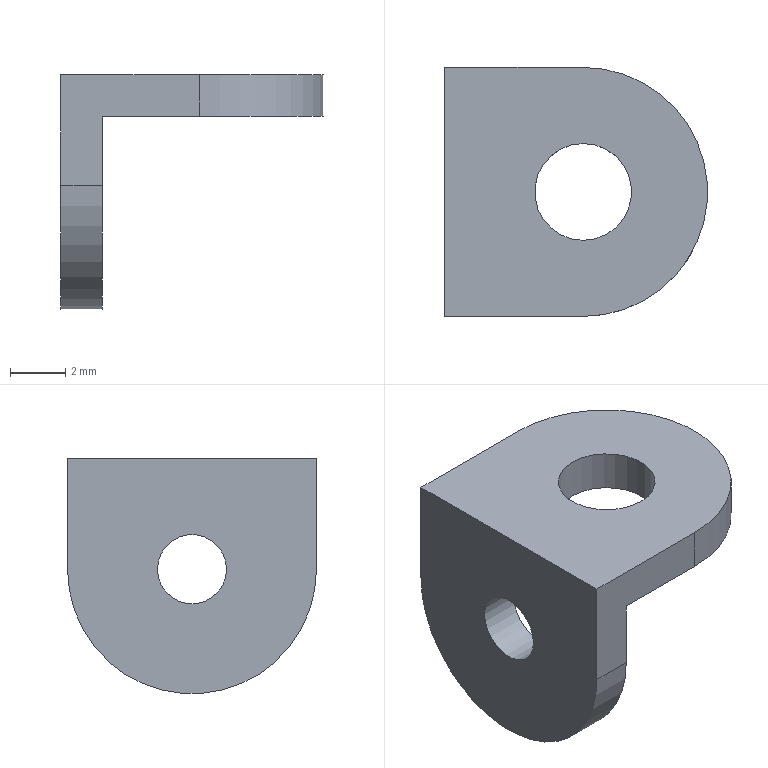Part | STEP file | 1-41.2 | 1 solid | 10 faces | box 9.5 x 9 x 8.5 mm | volume 174.881 mm3 | plane 6 | cylinder 4 | commonest cylinder face diameters 9 x2 2.5 x1 3.5 x1
STEP:
#1=CARTESIAN_POINT('',(0.,0.,0.));
#2=DIRECTION('',(0.,0.,1.));
#3=DIRECTION('',(1.,0.,0.));
#4=AXIS2_PLACEMENT_3D('',#1,#2,#3);
#5=CARTESIAN_POINT('',(0.,-4.5,1.5));
#6=VERTEX_POINT('',#5);
#7=CARTESIAN_POINT('',(0.,4.5,1.5));
#8=VERTEX_POINT('',#7);
#9=CARTESIAN_POINT('',(0.,0.,1.5));
#10=DIRECTION('',(0.,0.,1.));
#11=DIRECTION('',(0.,-1.,0.));
#12=AXIS2_PLACEMENT_3D('',#9,#10,#11);
#13=CIRCLE('',#12,4.5);
#14=CARTESIAN_POINT('',(-0.25,0.25,1.5));
#15=DIRECTION('',(0.,0.,1.));
#16=DIRECTION('',(0.,1.,0.));
#17=AXIS2_PLACEMENT_3D('',#14,#15,#16);
#18=PLANE('',#17);
#19=CARTESIAN_POINT('',(-0.25,-0.25));
#20=DIRECTION('',(-1.,0.));
#21=AXIS2_PLACEMENT_2D('',#19,#20);
#22=CIRCLE('',#21,4.5);
#23=(GEOMETRIC_REPRESENTATION_CONTEXT(2)PARAMETRIC_REPRESENTATION_CONTEXT()REPRESENTATION_CONTEXT('',''));
#24=DEFINITIONAL_REPRESENTATION('',(#22),#23);
#25=PCURVE('',#18,#24);
#26=CARTESIAN_POINT('',(0.,0.,0.));
#27=DIRECTION('',(0.,0.,1.));
#28=DIRECTION('',(0.,-1.,0.));
#29=AXIS2_PLACEMENT_3D('',#26,#27,#28);
#30=CYLINDRICAL_SURFACE('',#29,4.5);
#31=CARTESIAN_POINT('',(0.,1.5));
#32=DIRECTION('',(1.,0.));
#33=VECTOR('',#32,1.);
#34=LINE('',#31,#33);
#35=(GEOMETRIC_REPRESENTATION_CONTEXT(2)PARAMETRIC_REPRESENTATION_CONTEXT()REPRESENTATION_CONTEXT('',''));
#36=DEFINITIONAL_REPRESENTATION('',(#34),#35);
#37=PCURVE('',#30,#36);
#38=SURFACE_CURVE('',#13,(#25,#37),.PCURVE_S1.);
#39=EDGE_CURVE('',#6,#8,#38,.T.);
#40=ORIENTED_EDGE('',*,*,#39,.T.);
#41=CARTESIAN_POINT('',(-5.,4.5,1.5));
#42=VERTEX_POINT('',#41);
#43=CARTESIAN_POINT('',(0.,4.5,1.5));
#44=DIRECTION('',(-1.,0.,0.));
#45=VECTOR('',#44,1.);
#46=LINE('',#43,#45);
#47=CARTESIAN_POINT('',(4.25,-0.25));
#48=DIRECTION('',(0.,1.));
#49=VECTOR('',#48,1.);
#50=LINE('',#47,#49);
#51=(GEOMETRIC_REPRESENTATION_CONTEXT(2)PARAMETRIC_REPRESENTATION_CONTEXT()REPRESENTATION_CONTEXT('',''));
#52=DEFINITIONAL_REPRESENTATION('',(#50),#51);
#53=PCURVE('',#18,#52);
#54=CARTESIAN_POINT('',(-2.5,4.5,-0.5));
#55=DIRECTION('',(0.,1.,0.));
#56=DIRECTION('',(-1.,0.,0.));
#57=AXIS2_PLACEMENT_3D('',#54,#55,#56);
#58=PLANE('',#57);
#59=CARTESIAN_POINT('',(-2.5,2.));
#60=DIRECTION('',(1.,0.));
#61=VECTOR('',#60,1.);
#62=LINE('',#59,#61);
#63=(GEOMETRIC_REPRESENTATION_CONTEXT(2)PARAMETRIC_REPRESENTATION_CONTEXT()REPRESENTATION_CONTEXT('',''));
#64=DEFINITIONAL_REPRESENTATION('',(#62),#63);
#65=PCURVE('',#58,#64);
#66=SURFACE_CURVE('',#46,(#53,#65),.PCURVE_S1.);
#67=EDGE_CURVE('',#8,#42,#66,.T.);
#68=ORIENTED_EDGE('',*,*,#67,.T.);
#69=CARTESIAN_POINT('',(-5.,-4.5,1.5));
#70=VERTEX_POINT('',#69);
#71=CARTESIAN_POINT('',(-5.,4.5,1.5));
#72=DIRECTION('',(0.,-1.,0.));
#73=VECTOR('',#72,1.);
#74=LINE('',#71,#73);
#75=CARTESIAN_POINT('',(4.25,4.75));
#76=DIRECTION('',(-1.,0.));
#77=VECTOR('',#76,1.);
#78=LINE('',#75,#77);
#79=(GEOMETRIC_REPRESENTATION_CONTEXT(2)PARAMETRIC_REPRESENTATION_CONTEXT()REPRESENTATION_CONTEXT('',''));
#80=DEFINITIONAL_REPRESENTATION('',(#78),#79);
#81=PCURVE('',#18,#80);
#82=CARTESIAN_POINT('',(-5.,0.,-2.5));
#83=DIRECTION('',(-1.,0.,0.));
#84=DIRECTION('',(0.,-1.,0.));
#85=AXIS2_PLACEMENT_3D('',#82,#83,#84);
#86=PLANE('',#85);
#87=CARTESIAN_POINT('',(-4.5,4.));
#88=DIRECTION('',(1.,0.));
#89=VECTOR('',#88,1.);
#90=LINE('',#87,#89);
#91=(GEOMETRIC_REPRESENTATION_CONTEXT(2)PARAMETRIC_REPRESENTATION_CONTEXT()REPRESENTATION_CONTEXT('',''));
#92=DEFINITIONAL_REPRESENTATION('',(#90),#91);
#93=PCURVE('',#86,#92);
#94=SURFACE_CURVE('',#74,(#81,#93),.PCURVE_S1.);
#95=EDGE_CURVE('',#42,#70,#94,.T.);
#96=ORIENTED_EDGE('',*,*,#95,.T.);
#97=CARTESIAN_POINT('',(-5.,-4.5,1.5));
#98=DIRECTION('',(1.,0.,0.));
#99=VECTOR('',#98,1.);
#100=LINE('',#97,#99);
#101=CARTESIAN_POINT('',(-4.75,4.75));
#102=DIRECTION('',(0.,-1.));
#103=VECTOR('',#102,1.);
#104=LINE('',#101,#103);
#105=(GEOMETRIC_REPRESENTATION_CONTEXT(2)PARAMETRIC_REPRESENTATION_CONTEXT()REPRESENTATION_CONTEXT('',''));
#106=DEFINITIONAL_REPRESENTATION('',(#104),#105);
#107=PCURVE('',#18,#106);
#108=CARTESIAN_POINT('',(-2.5,-4.5,-0.5));
#109=DIRECTION('',(0.,-1.,0.));
#110=DIRECTION('',(1.,0.,0.));
#111=AXIS2_PLACEMENT_3D('',#108,#109,#110);
#112=PLANE('',#111);
#113=CARTESIAN_POINT('',(-2.5,2.));
#114=DIRECTION('',(1.,0.));
#115=VECTOR('',#114,1.);
#116=LINE('',#113,#115);
#117=(GEOMETRIC_REPRESENTATION_CONTEXT(2)PARAMETRIC_REPRESENTATION_CONTEXT()REPRESENTATION_CONTEXT('',''));
#118=DEFINITIONAL_REPRESENTATION('',(#116),#117);
#119=PCURVE('',#112,#118);
#120=SURFACE_CURVE('',#100,(#107,#119),.PCURVE_S1.);
#121=EDGE_CURVE('',#70,#6,#120,.T.);
#122=ORIENTED_EDGE('',*,*,#121,.T.);
#123=EDGE_LOOP('',(#40,#68,#96,#122));
#124=FACE_BOUND('',#123,.T.);
#125=CARTESIAN_POINT('',(0.,1.75,1.5));
#126=VERTEX_POINT('',#125);
#127=CARTESIAN_POINT('',(0.,0.,1.5));
#128=DIRECTION('',(0.,0.,-1.));
#129=DIRECTION('',(0.,1.,0.));
#130=AXIS2_PLACEMENT_3D('',#127,#128,#129);
#131=CIRCLE('',#130,1.75);
#132=CARTESIAN_POINT('',(1.5,-0.25));
#133=CARTESIAN_POINT('',(1.5,-3.281));
#134=CARTESIAN_POINT('',(-1.125,-1.766));
#135=CARTESIAN_POINT('',(-3.75,-0.25));
#136=CARTESIAN_POINT('',(-1.125,1.266));
#137=CARTESIAN_POINT('',(1.5,2.781));
#138=CARTESIAN_POINT('',(1.5,-0.25));
#139=(BOUNDED_CURVE()B_SPLINE_CURVE(2,(#132,#133,#134,#135,#136,#137,#138),.UNSPECIFIED.,.T.,.F.)B_SPLINE_CURVE_WITH_KNOTS((1,2,2,2,2,1),(-2.094,0.,2.094,4.189,6.283,8.378),.UNSPECIFIED.)CURVE()GEOMETRIC_REPRESENTATION_ITEM()RATIONAL_B_SPLINE_CURVE((1.,0.5,1.,0.5,1.,0.5,1.))REPRESENTATION_ITEM(''));
#140=(GEOMETRIC_REPRESENTATION_CONTEXT(2)PARAMETRIC_REPRESENTATION_CONTEXT()REPRESENTATION_CONTEXT('',''));
#141=DEFINITIONAL_REPRESENTATION('',(#139),#140);
#142=PCURVE('',#18,#141);
#143=CARTESIAN_POINT('',(0.,0.,0.));
#144=DIRECTION('',(0.,0.,1.));
#145=DIRECTION('',(0.,1.,0.));
#146=AXIS2_PLACEMENT_3D('',#143,#144,#145);
#147=CYLINDRICAL_SURFACE('',#146,1.75);
#148=CARTESIAN_POINT('',(6.283,1.5));
#149=DIRECTION('',(-1.,0.));
#150=VECTOR('',#149,1.);
#151=LINE('',#148,#150);
#152=(GEOMETRIC_REPRESENTATION_CONTEXT(2)PARAMETRIC_REPRESENTATION_CONTEXT()REPRESENTATION_CONTEXT('',''));
#153=DEFINITIONAL_REPRESENTATION('',(#151),#152);
#154=PCURVE('',#147,#153);
#155=SURFACE_CURVE('',#131,(#142,#154),.PCURVE_S1.);
#156=EDGE_CURVE('',#126,#126,#155,.T.);
#157=ORIENTED_EDGE('',*,*,#156,.T.);
#158=EDGE_LOOP('',(#157));
#159=FACE_BOUND('',#158,.T.);
#160=ADVANCED_FACE('',(#124,#159),#18,.T.);
#161=CARTESIAN_POINT('',(0.,-4.5,0.));
#162=VERTEX_POINT('',#161);
#163=CARTESIAN_POINT('',(0.,4.5,0.));
#164=VERTEX_POINT('',#163);
#165=CARTESIAN_POINT('',(0.,0.,0.));
#166=DIRECTION('',(0.,0.,1.));
#167=DIRECTION('',(0.,-1.,0.));
#168=AXIS2_PLACEMENT_3D('',#165,#166,#167);
#169=CIRCLE('',#168,4.5);
#170=CARTESIAN_POINT('',(0.,0.));
#171=DIRECTION('',(1.,0.));
#172=VECTOR('',#171,1.);
#173=LINE('',#170,#172);
#174=(GEOMETRIC_REPRESENTATION_CONTEXT(2)PARAMETRIC_REPRESENTATION_CONTEXT()REPRESENTATION_CONTEXT('',''));
#175=DEFINITIONAL_REPRESENTATION('',(#173),#174);
#176=PCURVE('',#30,#175);
#177=CARTESIAN_POINT('',(-0.25,0.25,0.));
#178=DIRECTION('',(0.,0.,1.));
#179=DIRECTION('',(0.,1.,0.));
#180=AXIS2_PLACEMENT_3D('',#177,#178,#179);
#181=PLANE('',#180);
#182=CARTESIAN_POINT('',(-0.25,-0.25));
#183=DIRECTION('',(-1.,0.));
#184=AXIS2_PLACEMENT_2D('',#182,#183);
#185=CIRCLE('',#184,4.5);
#186=(GEOMETRIC_REPRESENTATION_CONTEXT(2)PARAMETRIC_REPRESENTATION_CONTEXT()REPRESENTATION_CONTEXT('',''));
#187=DEFINITIONAL_REPRESENTATION('',(#185),#186);
#188=PCURVE('',#181,#187);
#189=SURFACE_CURVE('',#169,(#176,#188),.PCURVE_S1.);
#190=EDGE_CURVE('',#162,#164,#189,.T.);
#191=ORIENTED_EDGE('',*,*,#190,.T.);
#192=CARTESIAN_POINT('',(0.,4.5,0.));
#193=DIRECTION('',(0.,0.,1.));
#194=VECTOR('',#193,1.);
#195=LINE('',#192,#194);
#196=CARTESIAN_POINT('',(3.142,0.));
#197=DIRECTION('',(0.,1.));
#198=VECTOR('',#197,1.);
#199=LINE('',#196,#198);
#200=(GEOMETRIC_REPRESENTATION_CONTEXT(2)PARAMETRIC_REPRESENTATION_CONTEXT()REPRESENTATION_CONTEXT('',''));
#201=DEFINITIONAL_REPRESENTATION('',(#199),#200);
#202=PCURVE('',#30,#201);
#203=CARTESIAN_POINT('',(-2.5,0.5));
#204=DIRECTION('',(0.,1.));
#205=VECTOR('',#204,1.);
#206=LINE('',#203,#205);
#207=(GEOMETRIC_REPRESENTATION_CONTEXT(2)PARAMETRIC_REPRESENTATION_CONTEXT()REPRESENTATION_CONTEXT('',''));
#208=DEFINITIONAL_REPRESENTATION('',(#206),#207);
#209=PCURVE('',#58,#208);
#210=SURFACE_CURVE('',#195,(#202,#209),.PCURVE_S1.);
#211=EDGE_CURVE('',#164,#8,#210,.T.);
#212=ORIENTED_EDGE('',*,*,#211,.T.);
#213=ORIENTED_EDGE('',*,*,#39,.F.);
#214=CARTESIAN_POINT('',(0.,-4.5,0.));
#215=DIRECTION('',(0.,0.,1.));
#216=VECTOR('',#215,1.);
#217=LINE('',#214,#216);
#218=CARTESIAN_POINT('',(0.,0.));
#219=DIRECTION('',(0.,1.));
#220=VECTOR('',#219,1.);
#221=LINE('',#218,#220);
#222=(GEOMETRIC_REPRESENTATION_CONTEXT(2)PARAMETRIC_REPRESENTATION_CONTEXT()REPRESENTATION_CONTEXT('',''));
#223=DEFINITIONAL_REPRESENTATION('',(#221),#222);
#224=PCURVE('',#30,#223);
#225=CARTESIAN_POINT('',(2.5,0.5));
#226=DIRECTION('',(0.,1.));
#227=VECTOR('',#226,1.);
#228=LINE('',#225,#227);
#229=(GEOMETRIC_REPRESENTATION_CONTEXT(2)PARAMETRIC_REPRESENTATION_CONTEXT()REPRESENTATION_CONTEXT('',''));
#230=DEFINITIONAL_REPRESENTATION('',(#228),#229);
#231=PCURVE('',#112,#230);
#232=SURFACE_CURVE('',#217,(#224,#231),.PCURVE_S1.);
#233=EDGE_CURVE('',#162,#6,#232,.T.);
#234=ORIENTED_EDGE('',*,*,#233,.F.);
#235=EDGE_LOOP('',(#191,#212,#213,#234));
#236=FACE_BOUND('',#235,.T.);
#237=ADVANCED_FACE('',(#236),#30,.T.);
#238=ORIENTED_EDGE('',*,*,#67,.F.);
#239=ORIENTED_EDGE('',*,*,#211,.F.);
#240=CARTESIAN_POINT('',(-3.5,4.5,0.));
#241=VERTEX_POINT('',#240);
#242=CARTESIAN_POINT('',(0.,4.5,0.));
#243=DIRECTION('',(-1.,0.,0.));
#244=VECTOR('',#243,1.);
#245=LINE('',#242,#244);
#246=CARTESIAN_POINT('',(-2.5,0.5));
#247=DIRECTION('',(1.,0.));
#248=VECTOR('',#247,1.);
#249=LINE('',#246,#248);
#250=(GEOMETRIC_REPRESENTATION_CONTEXT(2)PARAMETRIC_REPRESENTATION_CONTEXT()REPRESENTATION_CONTEXT('',''));
#251=DEFINITIONAL_REPRESENTATION('',(#249),#250);
#252=PCURVE('',#58,#251);
#253=CARTESIAN_POINT('',(4.25,-0.25));
#254=DIRECTION('',(0.,1.));
#255=VECTOR('',#254,1.);
#256=LINE('',#253,#255);
#257=(GEOMETRIC_REPRESENTATION_CONTEXT(2)PARAMETRIC_REPRESENTATION_CONTEXT()REPRESENTATION_CONTEXT('',''));
#258=DEFINITIONAL_REPRESENTATION('',(#256),#257);
#259=PCURVE('',#181,#258);
#260=SURFACE_CURVE('',#245,(#252,#259),.PCURVE_S1.);
#261=EDGE_CURVE('',#164,#241,#260,.T.);
#262=ORIENTED_EDGE('',*,*,#261,.T.);
#263=CARTESIAN_POINT('',(-3.5,4.5,-2.5));
#264=VERTEX_POINT('',#263);
#265=CARTESIAN_POINT('',(-3.5,4.5,0.));
#266=DIRECTION('',(0.,0.,-1.));
#267=VECTOR('',#266,1.);
#268=LINE('',#265,#267);
#269=CARTESIAN_POINT('',(1.,0.5));
#270=DIRECTION('',(0.,-1.));
#271=VECTOR('',#270,1.);
#272=LINE('',#269,#271);
#273=(GEOMETRIC_REPRESENTATION_CONTEXT(2)PARAMETRIC_REPRESENTATION_CONTEXT()REPRESENTATION_CONTEXT('',''));
#274=DEFINITIONAL_REPRESENTATION('',(#272),#273);
#275=PCURVE('',#58,#274);
#276=CARTESIAN_POINT('',(-3.5,0.,-2.5));
#277=DIRECTION('',(-1.,0.,0.));
#278=DIRECTION('',(0.,-1.,0.));
#279=AXIS2_PLACEMENT_3D('',#276,#277,#278);
#280=PLANE('',#279);
#281=CARTESIAN_POINT('',(-4.5,2.5));
#282=DIRECTION('',(0.,-1.));
#283=VECTOR('',#282,1.);
#284=LINE('',#281,#283);
#285=(GEOMETRIC_REPRESENTATION_CONTEXT(2)PARAMETRIC_REPRESENTATION_CONTEXT()REPRESENTATION_CONTEXT('',''));
#286=DEFINITIONAL_REPRESENTATION('',(#284),#285);
#287=PCURVE('',#280,#286);
#288=SURFACE_CURVE('',#268,(#275,#287),.PCURVE_S1.);
#289=EDGE_CURVE('',#241,#264,#288,.T.);
#290=ORIENTED_EDGE('',*,*,#289,.T.);
#291=CARTESIAN_POINT('',(-5.,4.5,-2.5));
#292=VERTEX_POINT('',#291);
#293=CARTESIAN_POINT('',(-5.,4.5,-2.5));
#294=DIRECTION('',(1.,0.,0.));
#295=VECTOR('',#294,1.);
#296=LINE('',#293,#295);
#297=CARTESIAN_POINT('',(2.5,-2.));
#298=DIRECTION('',(-1.,0.));
#299=VECTOR('',#298,1.);
#300=LINE('',#297,#299);
#301=(GEOMETRIC_REPRESENTATION_CONTEXT(2)PARAMETRIC_REPRESENTATION_CONTEXT()REPRESENTATION_CONTEXT('',''));
#302=DEFINITIONAL_REPRESENTATION('',(#300),#301);
#303=PCURVE('',#58,#302);
#304=CARTESIAN_POINT('',(-5.,0.,-2.5));
#305=DIRECTION('',(1.,0.,0.));
#306=DIRECTION('',(0.,1.,0.));
#307=AXIS2_PLACEMENT_3D('',#304,#305,#306);
#308=CYLINDRICAL_SURFACE('',#307,4.5);
#309=CARTESIAN_POINT('',(6.283,0.));
#310=DIRECTION('',(0.,1.));
#311=VECTOR('',#310,1.);
#312=LINE('',#309,#311);
#313=(GEOMETRIC_REPRESENTATION_CONTEXT(2)PARAMETRIC_REPRESENTATION_CONTEXT()REPRESENTATION_CONTEXT('',''));
#314=DEFINITIONAL_REPRESENTATION('',(#312),#313);
#315=PCURVE('',#308,#314);
#316=SURFACE_CURVE('',#296,(#303,#315),.PCURVE_S1.);
#317=EDGE_CURVE('',#292,#264,#316,.T.);
#318=ORIENTED_EDGE('',*,*,#317,.F.);
#319=CARTESIAN_POINT('',(-5.,4.5,-2.5));
#320=DIRECTION('',(0.,0.,1.));
#321=VECTOR('',#320,1.);
#322=LINE('',#319,#321);
#323=CARTESIAN_POINT('',(2.5,-2.));
#324=DIRECTION('',(0.,1.));
#325=VECTOR('',#324,1.);
#326=LINE('',#323,#325);
#327=(GEOMETRIC_REPRESENTATION_CONTEXT(2)PARAMETRIC_REPRESENTATION_CONTEXT()REPRESENTATION_CONTEXT('',''));
#328=DEFINITIONAL_REPRESENTATION('',(#326),#327);
#329=PCURVE('',#58,#328);
#330=CARTESIAN_POINT('',(-4.5,0.));
#331=DIRECTION('',(0.,1.));
#332=VECTOR('',#331,1.);
#333=LINE('',#330,#332);
#334=(GEOMETRIC_REPRESENTATION_CONTEXT(2)PARAMETRIC_REPRESENTATION_CONTEXT()REPRESENTATION_CONTEXT('',''));
#335=DEFINITIONAL_REPRESENTATION('',(#333),#334);
#336=PCURVE('',#86,#335);
#337=SURFACE_CURVE('',#322,(#329,#336),.PCURVE_S1.);
#338=EDGE_CURVE('',#292,#42,#337,.T.);
#339=ORIENTED_EDGE('',*,*,#338,.T.);
#340=EDGE_LOOP('',(#238,#239,#262,#290,#318,#339));
#341=FACE_BOUND('',#340,.T.);
#342=ADVANCED_FACE('',(#341),#58,.T.);
#343=ORIENTED_EDGE('',*,*,#95,.F.);
#344=ORIENTED_EDGE('',*,*,#338,.F.);
#345=CARTESIAN_POINT('',(-5.,-4.5,-2.5));
#346=VERTEX_POINT('',#345);
#347=CARTESIAN_POINT('',(-5.,0.,-2.5));
#348=DIRECTION('',(-1.,0.,0.));
#349=DIRECTION('',(0.,1.,0.));
#350=AXIS2_PLACEMENT_3D('',#347,#348,#349);
#351=CIRCLE('',#350,4.5);
#352=CARTESIAN_POINT('',(0.,0.));
#353=DIRECTION('',(-1.,0.));
#354=AXIS2_PLACEMENT_2D('',#352,#353);
#355=CIRCLE('',#354,4.5);
#356=(GEOMETRIC_REPRESENTATION_CONTEXT(2)PARAMETRIC_REPRESENTATION_CONTEXT()REPRESENTATION_CONTEXT('',''));
#357=DEFINITIONAL_REPRESENTATION('',(#355),#356);
#358=PCURVE('',#86,#357);
#359=CARTESIAN_POINT('',(6.283,0.));
#360=DIRECTION('',(-1.,0.));
#361=VECTOR('',#360,1.);
#362=LINE('',#359,#361);
#363=(GEOMETRIC_REPRESENTATION_CONTEXT(2)PARAMETRIC_REPRESENTATION_CONTEXT()REPRESENTATION_CONTEXT('',''));
#364=DEFINITIONAL_REPRESENTATION('',(#362),#363);
#365=PCURVE('',#308,#364);
#366=SURFACE_CURVE('',#351,(#358,#365),.PCURVE_S1.);
#367=EDGE_CURVE('',#292,#346,#366,.T.);
#368=ORIENTED_EDGE('',*,*,#367,.T.);
#369=CARTESIAN_POINT('',(-5.,-4.5,1.5));
#370=DIRECTION('',(0.,0.,-1.));
#371=VECTOR('',#370,1.);
#372=LINE('',#369,#371);
#373=CARTESIAN_POINT('',(4.5,4.));
#374=DIRECTION('',(0.,-1.));
#375=VECTOR('',#374,1.);
#376=LINE('',#373,#375);
#377=(GEOMETRIC_REPRESENTATION_CONTEXT(2)PARAMETRIC_REPRESENTATION_CONTEXT()REPRESENTATION_CONTEXT('',''));
#378=DEFINITIONAL_REPRESENTATION('',(#376),#377);
#379=PCURVE('',#86,#378);
#380=CARTESIAN_POINT('',(-2.5,2.));
#381=DIRECTION('',(0.,-1.));
#382=VECTOR('',#381,1.);
#383=LINE('',#380,#382);
#384=(GEOMETRIC_REPRESENTATION_CONTEXT(2)PARAMETRIC_REPRESENTATION_CONTEXT()REPRESENTATION_CONTEXT('',''));
#385=DEFINITIONAL_REPRESENTATION('',(#383),#384);
#386=PCURVE('',#112,#385);
#387=SURFACE_CURVE('',#372,(#379,#386),.PCURVE_S1.);
#388=EDGE_CURVE('',#70,#346,#387,.T.);
#389=ORIENTED_EDGE('',*,*,#388,.F.);
#390=EDGE_LOOP('',(#343,#344,#368,#389));
#391=FACE_BOUND('',#390,.T.);
#392=CARTESIAN_POINT('',(-5.,-1.25,-2.5));
#393=VERTEX_POINT('',#392);
#394=CARTESIAN_POINT('',(-5.,0.,-2.5));
#395=DIRECTION('',(1.,0.,0.));
#396=DIRECTION('',(0.,-1.,0.));
#397=AXIS2_PLACEMENT_3D('',#394,#395,#396);
#398=CIRCLE('',#397,1.25);
#399=CARTESIAN_POINT('',(1.25,0.));
#400=CARTESIAN_POINT('',(1.25,-2.165));
#401=CARTESIAN_POINT('',(-0.625,-1.083));
#402=CARTESIAN_POINT('',(-2.5,0.));
#403=CARTESIAN_POINT('',(-0.625,1.083));
#404=CARTESIAN_POINT('',(1.25,2.165));
#405=CARTESIAN_POINT('',(1.25,0.));
#406=(BOUNDED_CURVE()B_SPLINE_CURVE(2,(#399,#400,#401,#402,#403,#404,#405),.UNSPECIFIED.,.T.,.F.)B_SPLINE_CURVE_WITH_KNOTS((1,2,2,2,2,1),(-2.094,0.,2.094,4.189,6.283,8.378),.UNSPECIFIED.)CURVE()GEOMETRIC_REPRESENTATION_ITEM()RATIONAL_B_SPLINE_CURVE((1.,0.5,1.,0.5,1.,0.5,1.))REPRESENTATION_ITEM(''));
#407=(GEOMETRIC_REPRESENTATION_CONTEXT(2)PARAMETRIC_REPRESENTATION_CONTEXT()REPRESENTATION_CONTEXT('',''));
#408=DEFINITIONAL_REPRESENTATION('',(#406),#407);
#409=PCURVE('',#86,#408);
#410=CARTESIAN_POINT('',(-5.,0.,-2.5));
#411=DIRECTION('',(1.,0.,0.));
#412=DIRECTION('',(0.,-1.,0.));
#413=AXIS2_PLACEMENT_3D('',#410,#411,#412);
#414=CYLINDRICAL_SURFACE('',#413,1.25);
#415=CARTESIAN_POINT('',(0.,0.));
#416=DIRECTION('',(1.,0.));
#417=VECTOR('',#416,1.);
#418=LINE('',#415,#417);
#419=(GEOMETRIC_REPRESENTATION_CONTEXT(2)PARAMETRIC_REPRESENTATION_CONTEXT()REPRESENTATION_CONTEXT('',''));
#420=DEFINITIONAL_REPRESENTATION('',(#418),#419);
#421=PCURVE('',#414,#420);
#422=SURFACE_CURVE('',#398,(#409,#421),.PCURVE_S1.);
#423=EDGE_CURVE('',#393,#393,#422,.T.);
#424=ORIENTED_EDGE('',*,*,#423,.T.);
#425=EDGE_LOOP('',(#424));
#426=FACE_BOUND('',#425,.T.);
#427=ADVANCED_FACE('',(#391,#426),#86,.T.);
#428=CARTESIAN_POINT('',(-3.5,-4.5,0.));
#429=VERTEX_POINT('',#428);
#430=CARTESIAN_POINT('',(-3.5,-4.5,0.));
#431=DIRECTION('',(1.,0.,0.));
#432=VECTOR('',#431,1.);
#433=LINE('',#430,#432);
#434=CARTESIAN_POINT('',(-1.,0.5));
#435=DIRECTION('',(1.,0.));
#436=VECTOR('',#435,1.);
#437=LINE('',#434,#436);
#438=(GEOMETRIC_REPRESENTATION_CONTEXT(2)PARAMETRIC_REPRESENTATION_CONTEXT()REPRESENTATION_CONTEXT('',''));
#439=DEFINITIONAL_REPRESENTATION('',(#437),#438);
#440=PCURVE('',#112,#439);
#441=CARTESIAN_POINT('',(-4.75,3.25));
#442=DIRECTION('',(0.,-1.));
#443=VECTOR('',#442,1.);
#444=LINE('',#441,#443);
#445=(GEOMETRIC_REPRESENTATION_CONTEXT(2)PARAMETRIC_REPRESENTATION_CONTEXT()REPRESENTATION_CONTEXT('',''));
#446=DEFINITIONAL_REPRESENTATION('',(#444),#445);
#447=PCURVE('',#181,#446);
#448=SURFACE_CURVE('',#433,(#440,#447),.PCURVE_S1.);
#449=EDGE_CURVE('',#429,#162,#448,.T.);
#450=ORIENTED_EDGE('',*,*,#449,.T.);
#451=ORIENTED_EDGE('',*,*,#233,.T.);
#452=ORIENTED_EDGE('',*,*,#121,.F.);
#453=ORIENTED_EDGE('',*,*,#388,.T.);
#454=CARTESIAN_POINT('',(-3.5,-4.5,-2.5));
#455=VERTEX_POINT('',#454);
#456=CARTESIAN_POINT('',(-5.,-4.5,-2.5));
#457=DIRECTION('',(1.,0.,0.));
#458=VECTOR('',#457,1.);
#459=LINE('',#456,#458);
#460=CARTESIAN_POINT('',(-2.5,-2.));
#461=DIRECTION('',(1.,0.));
#462=VECTOR('',#461,1.);
#463=LINE('',#460,#462);
#464=(GEOMETRIC_REPRESENTATION_CONTEXT(2)PARAMETRIC_REPRESENTATION_CONTEXT()REPRESENTATION_CONTEXT('',''));
#465=DEFINITIONAL_REPRESENTATION('',(#463),#464);
#466=PCURVE('',#112,#465);
#467=CARTESIAN_POINT('',(3.142,0.));
#468=DIRECTION('',(0.,1.));
#469=VECTOR('',#468,1.);
#470=LINE('',#467,#469);
#471=(GEOMETRIC_REPRESENTATION_CONTEXT(2)PARAMETRIC_REPRESENTATION_CONTEXT()REPRESENTATION_CONTEXT('',''));
#472=DEFINITIONAL_REPRESENTATION('',(#470),#471);
#473=PCURVE('',#308,#472);
#474=SURFACE_CURVE('',#459,(#466,#473),.PCURVE_S1.);
#475=EDGE_CURVE('',#346,#455,#474,.T.);
#476=ORIENTED_EDGE('',*,*,#475,.T.);
#477=CARTESIAN_POINT('',(-3.5,-4.5,-2.5));
#478=DIRECTION('',(0.,0.,1.));
#479=VECTOR('',#478,1.);
#480=LINE('',#477,#479);
#481=CARTESIAN_POINT('',(-1.,-2.));
#482=DIRECTION('',(0.,1.));
#483=VECTOR('',#482,1.);
#484=LINE('',#481,#483);
#485=(GEOMETRIC_REPRESENTATION_CONTEXT(2)PARAMETRIC_REPRESENTATION_CONTEXT()REPRESENTATION_CONTEXT('',''));
#486=DEFINITIONAL_REPRESENTATION('',(#484),#485);
#487=PCURVE('',#112,#486);
#488=CARTESIAN_POINT('',(4.5,0.));
#489=DIRECTION('',(0.,1.));
#490=VECTOR('',#489,1.);
#491=LINE('',#488,#490);
#492=(GEOMETRIC_REPRESENTATION_CONTEXT(2)PARAMETRIC_REPRESENTATION_CONTEXT()REPRESENTATION_CONTEXT('',''));
#493=DEFINITIONAL_REPRESENTATION('',(#491),#492);
#494=PCURVE('',#280,#493);
#495=SURFACE_CURVE('',#480,(#487,#494),.PCURVE_S1.);
#496=EDGE_CURVE('',#455,#429,#495,.T.);
#497=ORIENTED_EDGE('',*,*,#496,.T.);
#498=EDGE_LOOP('',(#450,#451,#452,#453,#476,#497));
#499=FACE_BOUND('',#498,.T.);
#500=ADVANCED_FACE('',(#499),#112,.T.);
#501=CARTESIAN_POINT('',(0.,1.75,0.));
#502=VERTEX_POINT('',#501);
#503=CARTESIAN_POINT('',(0.,1.75,0.));
#504=DIRECTION('',(0.,0.,1.));
#505=VECTOR('',#504,1.);
#506=LINE('',#503,#505);
#507=CARTESIAN_POINT('',(6.283,0.));
#508=DIRECTION('',(0.,1.));
#509=VECTOR('',#508,1.);
#510=LINE('',#507,#509);
#511=(GEOMETRIC_REPRESENTATION_CONTEXT(2)PARAMETRIC_REPRESENTATION_CONTEXT()REPRESENTATION_CONTEXT('',''));
#512=DEFINITIONAL_REPRESENTATION('',(#510),#511);
#513=PCURVE('',#147,#512);
#514=CARTESIAN_POINT('',(0.,0.));
#515=DIRECTION('',(0.,1.));
#516=VECTOR('',#515,1.);
#517=LINE('',#514,#516);
#518=(GEOMETRIC_REPRESENTATION_CONTEXT(2)PARAMETRIC_REPRESENTATION_CONTEXT()REPRESENTATION_CONTEXT('',''));
#519=DEFINITIONAL_REPRESENTATION('',(#517),#518);
#520=PCURVE('',#147,#519);
#521=SEAM_CURVE('',#506,(#513,#520),.PCURVE_S1.);
#522=EDGE_CURVE('',#502,#126,#521,.T.);
#523=ORIENTED_EDGE('',*,*,#522,.T.);
#524=ORIENTED_EDGE('',*,*,#156,.T.);
#525=ORIENTED_EDGE('',*,*,#522,.F.);
#526=CARTESIAN_POINT('',(0.,0.,0.));
#527=DIRECTION('',(0.,0.,-1.));
#528=DIRECTION('',(0.,1.,0.));
#529=AXIS2_PLACEMENT_3D('',#526,#527,#528);
#530=CIRCLE('',#529,1.75);
#531=CARTESIAN_POINT('',(6.283,0.));
#532=DIRECTION('',(-1.,0.));
#533=VECTOR('',#532,1.);
#534=LINE('',#531,#533);
#535=(GEOMETRIC_REPRESENTATION_CONTEXT(2)PARAMETRIC_REPRESENTATION_CONTEXT()REPRESENTATION_CONTEXT('',''));
#536=DEFINITIONAL_REPRESENTATION('',(#534),#535);
#537=PCURVE('',#147,#536);
#538=CARTESIAN_POINT('',(1.5,-0.25));
#539=CARTESIAN_POINT('',(1.5,-3.281));
#540=CARTESIAN_POINT('',(-1.125,-1.766));
#541=CARTESIAN_POINT('',(-3.75,-0.25));
#542=CARTESIAN_POINT('',(-1.125,1.266));
#543=CARTESIAN_POINT('',(1.5,2.781));
#544=CARTESIAN_POINT('',(1.5,-0.25));
#545=(BOUNDED_CURVE()B_SPLINE_CURVE(2,(#538,#539,#540,#541,#542,#543,#544),.UNSPECIFIED.,.T.,.F.)B_SPLINE_CURVE_WITH_KNOTS((1,2,2,2,2,1),(-2.094,0.,2.094,4.189,6.283,8.378),.UNSPECIFIED.)CURVE()GEOMETRIC_REPRESENTATION_ITEM()RATIONAL_B_SPLINE_CURVE((1.,0.5,1.,0.5,1.,0.5,1.))REPRESENTATION_ITEM(''));
#546=(GEOMETRIC_REPRESENTATION_CONTEXT(2)PARAMETRIC_REPRESENTATION_CONTEXT()REPRESENTATION_CONTEXT('',''));
#547=DEFINITIONAL_REPRESENTATION('',(#545),#546);
#548=PCURVE('',#181,#547);
#549=SURFACE_CURVE('',#530,(#537,#548),.PCURVE_S1.);
#550=EDGE_CURVE('',#502,#502,#549,.T.);
#551=ORIENTED_EDGE('',*,*,#550,.F.);
#552=EDGE_LOOP('',(#523,#524,#525,#551));
#553=FACE_BOUND('',#552,.F.);
#554=ADVANCED_FACE('',(#553),#147,.F.);
#555=ORIENTED_EDGE('',*,*,#190,.T.);
#556=ORIENTED_EDGE('',*,*,#261,.T.);
#557=CARTESIAN_POINT('',(-3.5,-4.5,0.));
#558=DIRECTION('',(0.,1.,0.));
#559=VECTOR('',#558,1.);
#560=LINE('',#557,#559);
#561=CARTESIAN_POINT('',(-4.75,3.25));
#562=DIRECTION('',(1.,0.));
#563=VECTOR('',#562,1.);
#564=LINE('',#561,#563);
#565=(GEOMETRIC_REPRESENTATION_CONTEXT(2)PARAMETRIC_REPRESENTATION_CONTEXT()REPRESENTATION_CONTEXT('',''));
#566=DEFINITIONAL_REPRESENTATION('',(#564),#565);
#567=PCURVE('',#181,#566);
#568=CARTESIAN_POINT('',(4.5,2.5));
#569=DIRECTION('',(-1.,0.));
#570=VECTOR('',#569,1.);
#571=LINE('',#568,#570);
#572=(GEOMETRIC_REPRESENTATION_CONTEXT(2)PARAMETRIC_REPRESENTATION_CONTEXT()REPRESENTATION_CONTEXT('',''));
#573=DEFINITIONAL_REPRESENTATION('',(#571),#572);
#574=PCURVE('',#280,#573);
#575=SURFACE_CURVE('',#560,(#567,#574),.PCURVE_S1.);
#576=EDGE_CURVE('',#429,#241,#575,.T.);
#577=ORIENTED_EDGE('',*,*,#576,.F.);
#578=ORIENTED_EDGE('',*,*,#449,.T.);
#579=EDGE_LOOP('',(#555,#556,#577,#578));
#580=FACE_BOUND('',#579,.F.);
#581=ORIENTED_EDGE('',*,*,#550,.T.);
#582=EDGE_LOOP('',(#581));
#583=FACE_BOUND('',#582,.F.);
#584=ADVANCED_FACE('',(#580,#583),#181,.F.);
#585=CARTESIAN_POINT('',(-3.5,0.,-2.5));
#586=DIRECTION('',(-1.,0.,0.));
#587=DIRECTION('',(0.,1.,0.));
#588=AXIS2_PLACEMENT_3D('',#585,#586,#587);
#589=CIRCLE('',#588,4.5);
#590=CARTESIAN_POINT('',(0.,0.));
#591=DIRECTION('',(-1.,0.));
#592=AXIS2_PLACEMENT_2D('',#590,#591);
#593=CIRCLE('',#592,4.5);
#594=(GEOMETRIC_REPRESENTATION_CONTEXT(2)PARAMETRIC_REPRESENTATION_CONTEXT()REPRESENTATION_CONTEXT('',''));
#595=DEFINITIONAL_REPRESENTATION('',(#593),#594);
#596=PCURVE('',#280,#595);
#597=CARTESIAN_POINT('',(6.283,1.5));
#598=DIRECTION('',(-1.,0.));
#599=VECTOR('',#598,1.);
#600=LINE('',#597,#599);
#601=(GEOMETRIC_REPRESENTATION_CONTEXT(2)PARAMETRIC_REPRESENTATION_CONTEXT()REPRESENTATION_CONTEXT('',''));
#602=DEFINITIONAL_REPRESENTATION('',(#600),#601);
#603=PCURVE('',#308,#602);
#604=SURFACE_CURVE('',#589,(#596,#603),.PCURVE_S1.);
#605=EDGE_CURVE('',#264,#455,#604,.T.);
#606=ORIENTED_EDGE('',*,*,#605,.T.);
#607=ORIENTED_EDGE('',*,*,#496,.T.);
#608=ORIENTED_EDGE('',*,*,#576,.T.);
#609=ORIENTED_EDGE('',*,*,#289,.T.);
#610=EDGE_LOOP('',(#606,#607,#608,#609));
#611=FACE_BOUND('',#610,.F.);
#612=CARTESIAN_POINT('',(-3.5,-1.25,-2.5));
#613=VERTEX_POINT('',#612);
#614=CARTESIAN_POINT('',(-3.5,0.,-2.5));
#615=DIRECTION('',(1.,0.,0.));
#616=DIRECTION('',(0.,-1.,0.));
#617=AXIS2_PLACEMENT_3D('',#614,#615,#616);
#618=CIRCLE('',#617,1.25);
#619=CARTESIAN_POINT('',(1.25,0.));
#620=CARTESIAN_POINT('',(1.25,-2.165));
#621=CARTESIAN_POINT('',(-0.625,-1.083));
#622=CARTESIAN_POINT('',(-2.5,0.));
#623=CARTESIAN_POINT('',(-0.625,1.083));
#624=CARTESIAN_POINT('',(1.25,2.165));
#625=CARTESIAN_POINT('',(1.25,0.));
#626=(BOUNDED_CURVE()B_SPLINE_CURVE(2,(#619,#620,#621,#622,#623,#624,#625),.UNSPECIFIED.,.T.,.F.)B_SPLINE_CURVE_WITH_KNOTS((1,2,2,2,2,1),(-2.094,0.,2.094,4.189,6.283,8.378),.UNSPECIFIED.)CURVE()GEOMETRIC_REPRESENTATION_ITEM()RATIONAL_B_SPLINE_CURVE((1.,0.5,1.,0.5,1.,0.5,1.))REPRESENTATION_ITEM(''));
#627=(GEOMETRIC_REPRESENTATION_CONTEXT(2)PARAMETRIC_REPRESENTATION_CONTEXT()REPRESENTATION_CONTEXT('',''));
#628=DEFINITIONAL_REPRESENTATION('',(#626),#627);
#629=PCURVE('',#280,#628);
#630=CARTESIAN_POINT('',(0.,1.5));
#631=DIRECTION('',(1.,0.));
#632=VECTOR('',#631,1.);
#633=LINE('',#630,#632);
#634=(GEOMETRIC_REPRESENTATION_CONTEXT(2)PARAMETRIC_REPRESENTATION_CONTEXT()REPRESENTATION_CONTEXT('',''));
#635=DEFINITIONAL_REPRESENTATION('',(#633),#634);
#636=PCURVE('',#414,#635);
#637=SURFACE_CURVE('',#618,(#629,#636),.PCURVE_S1.);
#638=EDGE_CURVE('',#613,#613,#637,.T.);
#639=ORIENTED_EDGE('',*,*,#638,.T.);
#640=EDGE_LOOP('',(#639));
#641=FACE_BOUND('',#640,.F.);
#642=ADVANCED_FACE('',(#611,#641),#280,.F.);
#643=ORIENTED_EDGE('',*,*,#317,.T.);
#644=ORIENTED_EDGE('',*,*,#605,.T.);
#645=ORIENTED_EDGE('',*,*,#475,.F.);
#646=ORIENTED_EDGE('',*,*,#367,.F.);
#647=EDGE_LOOP('',(#643,#644,#645,#646));
#648=FACE_BOUND('',#647,.T.);
#649=ADVANCED_FACE('',(#648),#308,.T.);
#650=ORIENTED_EDGE('',*,*,#423,.T.);
#651=CARTESIAN_POINT('',(-5.,-1.25,-2.5));
#652=DIRECTION('',(1.,0.,0.));
#653=VECTOR('',#652,1.);
#654=LINE('',#651,#653);
#655=CARTESIAN_POINT('',(6.283,0.));
#656=DIRECTION('',(0.,1.));
#657=VECTOR('',#656,1.);
#658=LINE('',#655,#657);
#659=(GEOMETRIC_REPRESENTATION_CONTEXT(2)PARAMETRIC_REPRESENTATION_CONTEXT()REPRESENTATION_CONTEXT('',''));
#660=DEFINITIONAL_REPRESENTATION('',(#658),#659);
#661=PCURVE('',#414,#660);
#662=CARTESIAN_POINT('',(0.,0.));
#663=DIRECTION('',(0.,1.));
#664=VECTOR('',#663,1.);
#665=LINE('',#662,#664);
#666=(GEOMETRIC_REPRESENTATION_CONTEXT(2)PARAMETRIC_REPRESENTATION_CONTEXT()REPRESENTATION_CONTEXT('',''));
#667=DEFINITIONAL_REPRESENTATION('',(#665),#666);
#668=PCURVE('',#414,#667);
#669=SEAM_CURVE('',#654,(#661,#668),.PCURVE_S1.);
#670=EDGE_CURVE('',#393,#613,#669,.T.);
#671=ORIENTED_EDGE('',*,*,#670,.T.);
#672=ORIENTED_EDGE('',*,*,#638,.F.);
#673=ORIENTED_EDGE('',*,*,#670,.F.);
#674=EDGE_LOOP('',(#650,#671,#672,#673));
#675=FACE_BOUND('',#674,.F.);
#676=ADVANCED_FACE('',(#675),#414,.F.);
#677=CLOSED_SHELL('',(#160,#237,#342,#427,#500,#554,#584,#642,#649,#676));
#678=MANIFOLD_SOLID_BREP('',#677);
#679=(LENGTH_UNIT()NAMED_UNIT(*)SI_UNIT(.MILLI.,.METRE.));
#680=UNCERTAINTY_MEASURE_WITH_UNIT(LENGTH_MEASURE(0.0000001),#679,'','');
#681=(NAMED_UNIT(*)PLANE_ANGLE_UNIT()SI_UNIT($,.RADIAN.));
#682=(NAMED_UNIT(*)SI_UNIT($,.STERADIAN.)SOLID_ANGLE_UNIT());
#683=(GEOMETRIC_REPRESENTATION_CONTEXT(3)GLOBAL_UNCERTAINTY_ASSIGNED_CONTEXT((#680))GLOBAL_UNIT_ASSIGNED_CONTEXT((#679,#681,#682))REPRESENTATION_CONTEXT('',''));
#684=ADVANCED_BREP_SHAPE_REPRESENTATION('',(#4,#678),#683);